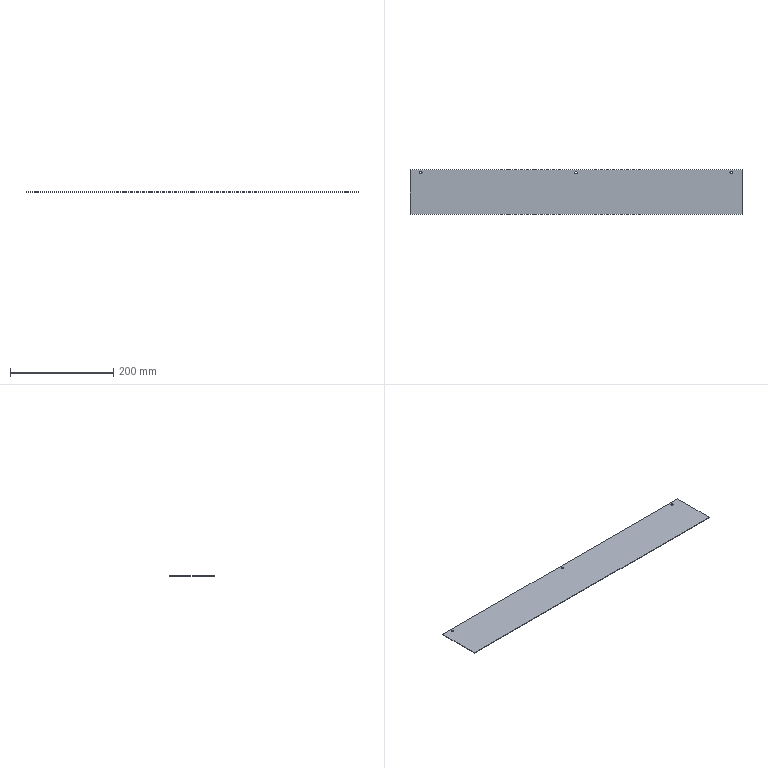Part | SolidWorks | features Cut 1, Extrusion 1 | 1 solid | 12 faces | box 642 x 87 x 1 mm | volume 55806 mm3 | cylinder 6 | plane 6 | commonest cylinder face diameters 4.5 x6
STEP:
#1=CARTESIAN_POINT('',(297.75,37.5,-0.5));
#2=VERTEX_POINT('',#1);
#3=CARTESIAN_POINT('',(302.25,37.5,-0.5));
#4=VERTEX_POINT('',#3);
#5=CARTESIAN_POINT('',(300.,37.5,-0.5));
#6=DIRECTION('',(0.,0.,1.));
#7=DIRECTION('',(-1.,0.,0.));
#8=AXIS2_PLACEMENT_3D('',#5,#6,#7);
#9=CIRCLE('',#8,2.25);
#10=EDGE_CURVE('',#2,#4,#9,.T.);
#11=ORIENTED_EDGE('',*,*,#10,.F.);
#12=CARTESIAN_POINT('',(297.75,37.5,0.5));
#13=VERTEX_POINT('',#12);
#14=CARTESIAN_POINT('',(297.75,37.5,-0.5));
#15=DIRECTION('',(0.,0.,1.));
#16=VECTOR('',#15,1000.);
#17=LINE('',#14,#16);
#18=EDGE_CURVE('',#2,#13,#17,.T.);
#19=ORIENTED_EDGE('',*,*,#18,.T.);
#20=CARTESIAN_POINT('',(302.25,37.5,0.5));
#21=VERTEX_POINT('',#20);
#22=CARTESIAN_POINT('',(300.,37.5,0.5));
#23=DIRECTION('',(0.,0.,1.));
#24=DIRECTION('',(-1.,0.,0.));
#25=AXIS2_PLACEMENT_3D('',#22,#23,#24);
#26=CIRCLE('',#25,2.25);
#27=EDGE_CURVE('',#13,#21,#26,.T.);
#28=ORIENTED_EDGE('',*,*,#27,.T.);
#29=CARTESIAN_POINT('',(302.25,37.5,-0.5));
#30=DIRECTION('',(0.,0.,1.));
#31=VECTOR('',#30,1000.);
#32=LINE('',#29,#31);
#33=EDGE_CURVE('',#4,#21,#32,.T.);
#34=ORIENTED_EDGE('',*,*,#33,.F.);
#35=EDGE_LOOP('',(#11,#19,#28,#34));
#36=FACE_OUTER_BOUND('',#35,.T.);
#37=CARTESIAN_POINT('',(300.,37.5,-0.5));
#38=DIRECTION('',(0.,0.,1.));
#39=DIRECTION('',(1.,0.,0.));
#40=AXIS2_PLACEMENT_3D('',#37,#38,#39);
#41=CYLINDRICAL_SURFACE('',#40,2.25);
#42=ADVANCED_FACE('',(#36),#41,.F.);
#43=CARTESIAN_POINT('',(-2.25,37.5,-0.5));
#44=VERTEX_POINT('',#43);
#45=CARTESIAN_POINT('',(2.25,37.5,-0.5));
#46=VERTEX_POINT('',#45);
#47=CARTESIAN_POINT('',(0.,37.5,-0.5));
#48=DIRECTION('',(0.,0.,1.));
#49=DIRECTION('',(1.,0.,0.));
#50=AXIS2_PLACEMENT_3D('',#47,#48,#49);
#51=CIRCLE('',#50,2.25);
#52=EDGE_CURVE('',#44,#46,#51,.T.);
#53=ORIENTED_EDGE('',*,*,#52,.F.);
#54=CARTESIAN_POINT('',(-2.25,37.5,0.5));
#55=VERTEX_POINT('',#54);
#56=CARTESIAN_POINT('',(-2.25,37.5,-0.5));
#57=DIRECTION('',(0.,0.,1.));
#58=VECTOR('',#57,1000.);
#59=LINE('',#56,#58);
#60=EDGE_CURVE('',#44,#55,#59,.T.);
#61=ORIENTED_EDGE('',*,*,#60,.T.);
#62=CARTESIAN_POINT('',(2.25,37.5,0.5));
#63=VERTEX_POINT('',#62);
#64=CARTESIAN_POINT('',(0.,37.5,0.5));
#65=DIRECTION('',(0.,0.,1.));
#66=DIRECTION('',(1.,0.,0.));
#67=AXIS2_PLACEMENT_3D('',#64,#65,#66);
#68=CIRCLE('',#67,2.25);
#69=EDGE_CURVE('',#55,#63,#68,.T.);
#70=ORIENTED_EDGE('',*,*,#69,.T.);
#71=CARTESIAN_POINT('',(2.25,37.5,-0.5));
#72=DIRECTION('',(0.,0.,1.));
#73=VECTOR('',#72,1000.);
#74=LINE('',#71,#73);
#75=EDGE_CURVE('',#46,#63,#74,.T.);
#76=ORIENTED_EDGE('',*,*,#75,.F.);
#77=EDGE_LOOP('',(#53,#61,#70,#76));
#78=FACE_OUTER_BOUND('',#77,.T.);
#79=CARTESIAN_POINT('',(0.,37.5,-0.5));
#80=DIRECTION('',(0.,0.,1.));
#81=DIRECTION('',(1.,0.,0.));
#82=AXIS2_PLACEMENT_3D('',#79,#80,#81);
#83=CYLINDRICAL_SURFACE('',#82,2.25);
#84=ADVANCED_FACE('',(#78),#83,.F.);
#85=CARTESIAN_POINT('',(-302.25,37.5,-0.5));
#86=VERTEX_POINT('',#85);
#87=CARTESIAN_POINT('',(-297.75,37.5,-0.5));
#88=VERTEX_POINT('',#87);
#89=CARTESIAN_POINT('',(-300.,37.5,-0.5));
#90=DIRECTION('',(0.,0.,1.));
#91=DIRECTION('',(1.,0.,0.));
#92=AXIS2_PLACEMENT_3D('',#89,#90,#91);
#93=CIRCLE('',#92,2.25);
#94=EDGE_CURVE('',#86,#88,#93,.T.);
#95=ORIENTED_EDGE('',*,*,#94,.F.);
#96=CARTESIAN_POINT('',(-302.25,37.5,0.5));
#97=VERTEX_POINT('',#96);
#98=CARTESIAN_POINT('',(-302.25,37.5,-0.5));
#99=DIRECTION('',(0.,0.,1.));
#100=VECTOR('',#99,1000.);
#101=LINE('',#98,#100);
#102=EDGE_CURVE('',#86,#97,#101,.T.);
#103=ORIENTED_EDGE('',*,*,#102,.T.);
#104=CARTESIAN_POINT('',(-297.75,37.5,0.5));
#105=VERTEX_POINT('',#104);
#106=CARTESIAN_POINT('',(-300.,37.5,0.5));
#107=DIRECTION('',(0.,0.,1.));
#108=DIRECTION('',(1.,0.,0.));
#109=AXIS2_PLACEMENT_3D('',#106,#107,#108);
#110=CIRCLE('',#109,2.25);
#111=EDGE_CURVE('',#97,#105,#110,.T.);
#112=ORIENTED_EDGE('',*,*,#111,.T.);
#113=CARTESIAN_POINT('',(-297.75,37.5,-0.5));
#114=DIRECTION('',(0.,0.,1.));
#115=VECTOR('',#114,1000.);
#116=LINE('',#113,#115);
#117=EDGE_CURVE('',#88,#105,#116,.T.);
#118=ORIENTED_EDGE('',*,*,#117,.F.);
#119=EDGE_LOOP('',(#95,#103,#112,#118));
#120=FACE_OUTER_BOUND('',#119,.T.);
#121=CARTESIAN_POINT('',(-300.,37.5,-0.5));
#122=DIRECTION('',(0.,0.,1.));
#123=DIRECTION('',(1.,0.,0.));
#124=AXIS2_PLACEMENT_3D('',#121,#122,#123);
#125=CYLINDRICAL_SURFACE('',#124,2.25);
#126=ADVANCED_FACE('',(#120),#125,.F.);
#127=CARTESIAN_POINT('',(-321.,-43.5,-0.5));
#128=VERTEX_POINT('',#127);
#129=CARTESIAN_POINT('',(-321.,-43.5,0.5));
#130=VERTEX_POINT('',#129);
#131=CARTESIAN_POINT('',(-321.,-43.5,-0.5));
#132=DIRECTION('',(0.,0.,1.));
#133=VECTOR('',#132,1000.);
#134=LINE('',#131,#133);
#135=EDGE_CURVE('',#128,#130,#134,.T.);
#136=ORIENTED_EDGE('',*,*,#135,.T.);
#137=CARTESIAN_POINT('',(-321.,43.5,0.5));
#138=VERTEX_POINT('',#137);
#139=CARTESIAN_POINT('',(-321.,43.5,0.5));
#140=DIRECTION('',(0.,-1.,0.));
#141=VECTOR('',#140,1000.);
#142=LINE('',#139,#141);
#143=EDGE_CURVE('',#138,#130,#142,.T.);
#144=ORIENTED_EDGE('',*,*,#143,.F.);
#145=CARTESIAN_POINT('',(-321.,43.5,-0.5));
#146=VERTEX_POINT('',#145);
#147=CARTESIAN_POINT('',(-321.,43.5,-0.5));
#148=DIRECTION('',(0.,0.,1.));
#149=VECTOR('',#148,1000.);
#150=LINE('',#147,#149);
#151=EDGE_CURVE('',#146,#138,#150,.T.);
#152=ORIENTED_EDGE('',*,*,#151,.F.);
#153=CARTESIAN_POINT('',(-321.,43.5,-0.5));
#154=DIRECTION('',(0.,-1.,0.));
#155=VECTOR('',#154,1000.);
#156=LINE('',#153,#155);
#157=EDGE_CURVE('',#146,#128,#156,.T.);
#158=ORIENTED_EDGE('',*,*,#157,.T.);
#159=EDGE_LOOP('',(#136,#144,#152,#158));
#160=FACE_OUTER_BOUND('',#159,.T.);
#161=CARTESIAN_POINT('',(-321.,43.5,-0.5));
#162=DIRECTION('',(1.,0.,0.));
#163=DIRECTION('',(0.,0.,-1.));
#164=AXIS2_PLACEMENT_3D('',#161,#162,#163);
#165=PLANE('',#164);
#166=ADVANCED_FACE('',(#160),#165,.F.);
#167=CARTESIAN_POINT('',(300.,37.5,0.5));
#168=DIRECTION('',(0.,0.,1.));
#169=DIRECTION('',(-1.,0.,0.));
#170=AXIS2_PLACEMENT_3D('',#167,#168,#169);
#171=CIRCLE('',#170,2.25);
#172=EDGE_CURVE('',#21,#13,#171,.T.);
#173=ORIENTED_EDGE('',*,*,#172,.F.);
#174=ORIENTED_EDGE('',*,*,#27,.F.);
#175=EDGE_LOOP('',(#173,#174));
#176=FACE_BOUND('',#175,.T.);
#177=CARTESIAN_POINT('',(0.,37.5,0.5));
#178=DIRECTION('',(0.,0.,1.));
#179=DIRECTION('',(1.,0.,0.));
#180=AXIS2_PLACEMENT_3D('',#177,#178,#179);
#181=CIRCLE('',#180,2.25);
#182=EDGE_CURVE('',#63,#55,#181,.T.);
#183=ORIENTED_EDGE('',*,*,#182,.F.);
#184=ORIENTED_EDGE('',*,*,#69,.F.);
#185=EDGE_LOOP('',(#183,#184));
#186=FACE_BOUND('',#185,.T.);
#187=CARTESIAN_POINT('',(-300.,37.5,0.5));
#188=DIRECTION('',(0.,0.,1.));
#189=DIRECTION('',(1.,0.,0.));
#190=AXIS2_PLACEMENT_3D('',#187,#188,#189);
#191=CIRCLE('',#190,2.25);
#192=EDGE_CURVE('',#105,#97,#191,.T.);
#193=ORIENTED_EDGE('',*,*,#192,.F.);
#194=ORIENTED_EDGE('',*,*,#111,.F.);
#195=EDGE_LOOP('',(#193,#194));
#196=FACE_BOUND('',#195,.T.);
#197=CARTESIAN_POINT('',(321.,-43.5,0.5));
#198=VERTEX_POINT('',#197);
#199=CARTESIAN_POINT('',(-321.,-43.5,0.5));
#200=DIRECTION('',(1.,0.,0.));
#201=VECTOR('',#200,1000.);
#202=LINE('',#199,#201);
#203=EDGE_CURVE('',#130,#198,#202,.T.);
#204=ORIENTED_EDGE('',*,*,#203,.T.);
#205=CARTESIAN_POINT('',(321.,43.5,0.5));
#206=VERTEX_POINT('',#205);
#207=CARTESIAN_POINT('',(321.,43.5,0.5));
#208=DIRECTION('',(0.,-1.,0.));
#209=VECTOR('',#208,1000.);
#210=LINE('',#207,#209);
#211=EDGE_CURVE('',#206,#198,#210,.T.);
#212=ORIENTED_EDGE('',*,*,#211,.F.);
#213=CARTESIAN_POINT('',(-321.,43.5,0.5));
#214=DIRECTION('',(1.,0.,0.));
#215=VECTOR('',#214,1000.);
#216=LINE('',#213,#215);
#217=EDGE_CURVE('',#138,#206,#216,.T.);
#218=ORIENTED_EDGE('',*,*,#217,.F.);
#219=ORIENTED_EDGE('',*,*,#143,.T.);
#220=EDGE_LOOP('',(#204,#212,#218,#219));
#221=FACE_OUTER_BOUND('',#220,.T.);
#222=CARTESIAN_POINT('',(-321.,43.5,0.5));
#223=DIRECTION('',(0.,0.,-1.));
#224=DIRECTION('',(-1.,0.,0.));
#225=AXIS2_PLACEMENT_3D('',#222,#223,#224);
#226=PLANE('',#225);
#227=ADVANCED_FACE('',(#176,#186,#196,#221),#226,.F.);
#228=CARTESIAN_POINT('',(321.,-43.5,-0.5));
#229=VERTEX_POINT('',#228);
#230=CARTESIAN_POINT('',(321.,-43.5,-0.5));
#231=DIRECTION('',(0.,0.,-1.));
#232=VECTOR('',#231,1000.);
#233=LINE('',#230,#232);
#234=EDGE_CURVE('',#198,#229,#233,.T.);
#235=ORIENTED_EDGE('',*,*,#234,.T.);
#236=CARTESIAN_POINT('',(321.,43.5,-0.5));
#237=VERTEX_POINT('',#236);
#238=CARTESIAN_POINT('',(321.,43.5,-0.5));
#239=DIRECTION('',(0.,-1.,0.));
#240=VECTOR('',#239,1000.);
#241=LINE('',#238,#240);
#242=EDGE_CURVE('',#237,#229,#241,.T.);
#243=ORIENTED_EDGE('',*,*,#242,.F.);
#244=CARTESIAN_POINT('',(321.,43.5,-0.5));
#245=DIRECTION('',(0.,0.,-1.));
#246=VECTOR('',#245,1000.);
#247=LINE('',#244,#246);
#248=EDGE_CURVE('',#206,#237,#247,.T.);
#249=ORIENTED_EDGE('',*,*,#248,.F.);
#250=ORIENTED_EDGE('',*,*,#211,.T.);
#251=EDGE_LOOP('',(#235,#243,#249,#250));
#252=FACE_OUTER_BOUND('',#251,.T.);
#253=CARTESIAN_POINT('',(321.,43.5,-0.5));
#254=DIRECTION('',(-1.,0.,0.));
#255=DIRECTION('',(0.,0.,1.));
#256=AXIS2_PLACEMENT_3D('',#253,#254,#255);
#257=PLANE('',#256);
#258=ADVANCED_FACE('',(#252),#257,.F.);
#259=CARTESIAN_POINT('',(300.,37.5,-0.5));
#260=DIRECTION('',(0.,0.,1.));
#261=DIRECTION('',(-1.,0.,0.));
#262=AXIS2_PLACEMENT_3D('',#259,#260,#261);
#263=CIRCLE('',#262,2.25);
#264=EDGE_CURVE('',#4,#2,#263,.T.);
#265=ORIENTED_EDGE('',*,*,#264,.T.);
#266=ORIENTED_EDGE('',*,*,#10,.T.);
#267=EDGE_LOOP('',(#265,#266));
#268=FACE_BOUND('',#267,.T.);
#269=CARTESIAN_POINT('',(0.,37.5,-0.5));
#270=DIRECTION('',(0.,0.,1.));
#271=DIRECTION('',(1.,0.,0.));
#272=AXIS2_PLACEMENT_3D('',#269,#270,#271);
#273=CIRCLE('',#272,2.25);
#274=EDGE_CURVE('',#46,#44,#273,.T.);
#275=ORIENTED_EDGE('',*,*,#274,.T.);
#276=ORIENTED_EDGE('',*,*,#52,.T.);
#277=EDGE_LOOP('',(#275,#276));
#278=FACE_BOUND('',#277,.T.);
#279=CARTESIAN_POINT('',(-300.,37.5,-0.5));
#280=DIRECTION('',(0.,0.,1.));
#281=DIRECTION('',(1.,0.,0.));
#282=AXIS2_PLACEMENT_3D('',#279,#280,#281);
#283=CIRCLE('',#282,2.25);
#284=EDGE_CURVE('',#88,#86,#283,.T.);
#285=ORIENTED_EDGE('',*,*,#284,.T.);
#286=ORIENTED_EDGE('',*,*,#94,.T.);
#287=EDGE_LOOP('',(#285,#286));
#288=FACE_BOUND('',#287,.T.);
#289=CARTESIAN_POINT('',(-321.,-43.5,-0.5));
#290=DIRECTION('',(-1.,0.,0.));
#291=VECTOR('',#290,1000.);
#292=LINE('',#289,#291);
#293=EDGE_CURVE('',#229,#128,#292,.T.);
#294=ORIENTED_EDGE('',*,*,#293,.T.);
#295=ORIENTED_EDGE('',*,*,#157,.F.);
#296=CARTESIAN_POINT('',(-321.,43.5,-0.5));
#297=DIRECTION('',(-1.,0.,0.));
#298=VECTOR('',#297,1000.);
#299=LINE('',#296,#298);
#300=EDGE_CURVE('',#237,#146,#299,.T.);
#301=ORIENTED_EDGE('',*,*,#300,.F.);
#302=ORIENTED_EDGE('',*,*,#242,.T.);
#303=EDGE_LOOP('',(#294,#295,#301,#302));
#304=FACE_OUTER_BOUND('',#303,.T.);
#305=CARTESIAN_POINT('',(-321.,43.5,-0.5));
#306=DIRECTION('',(0.,0.,1.));
#307=DIRECTION('',(1.,0.,0.));
#308=AXIS2_PLACEMENT_3D('',#305,#306,#307);
#309=PLANE('',#308);
#310=ADVANCED_FACE('',(#268,#278,#288,#304),#309,.F.);
#311=ORIENTED_EDGE('',*,*,#151,.T.);
#312=ORIENTED_EDGE('',*,*,#217,.T.);
#313=ORIENTED_EDGE('',*,*,#248,.T.);
#314=ORIENTED_EDGE('',*,*,#300,.T.);
#315=EDGE_LOOP('',(#311,#312,#313,#314));
#316=FACE_OUTER_BOUND('',#315,.T.);
#317=CARTESIAN_POINT('',(-321.,43.5,0.5));
#318=DIRECTION('',(0.,1.,0.));
#319=DIRECTION('',(0.,0.,1.));
#320=AXIS2_PLACEMENT_3D('',#317,#318,#319);
#321=PLANE('',#320);
#322=ADVANCED_FACE('',(#316),#321,.T.);
#323=ORIENTED_EDGE('',*,*,#135,.F.);
#324=ORIENTED_EDGE('',*,*,#293,.F.);
#325=ORIENTED_EDGE('',*,*,#234,.F.);
#326=ORIENTED_EDGE('',*,*,#203,.F.);
#327=EDGE_LOOP('',(#323,#324,#325,#326));
#328=FACE_OUTER_BOUND('',#327,.T.);
#329=CARTESIAN_POINT('',(-321.,-43.5,0.5));
#330=DIRECTION('',(0.,1.,0.));
#331=DIRECTION('',(0.,0.,1.));
#332=AXIS2_PLACEMENT_3D('',#329,#330,#331);
#333=PLANE('',#332);
#334=ADVANCED_FACE('',(#328),#333,.F.);
#335=ORIENTED_EDGE('',*,*,#102,.F.);
#336=ORIENTED_EDGE('',*,*,#284,.F.);
#337=ORIENTED_EDGE('',*,*,#117,.T.);
#338=ORIENTED_EDGE('',*,*,#192,.T.);
#339=EDGE_LOOP('',(#335,#336,#337,#338));
#340=FACE_OUTER_BOUND('',#339,.T.);
#341=CARTESIAN_POINT('',(-300.,37.5,-0.5));
#342=DIRECTION('',(0.,0.,1.));
#343=DIRECTION('',(1.,0.,0.));
#344=AXIS2_PLACEMENT_3D('',#341,#342,#343);
#345=CYLINDRICAL_SURFACE('',#344,2.25);
#346=ADVANCED_FACE('',(#340),#345,.F.);
#347=ORIENTED_EDGE('',*,*,#60,.F.);
#348=ORIENTED_EDGE('',*,*,#274,.F.);
#349=ORIENTED_EDGE('',*,*,#75,.T.);
#350=ORIENTED_EDGE('',*,*,#182,.T.);
#351=EDGE_LOOP('',(#347,#348,#349,#350));
#352=FACE_OUTER_BOUND('',#351,.T.);
#353=CARTESIAN_POINT('',(0.,37.5,-0.5));
#354=DIRECTION('',(0.,0.,1.));
#355=DIRECTION('',(1.,0.,0.));
#356=AXIS2_PLACEMENT_3D('',#353,#354,#355);
#357=CYLINDRICAL_SURFACE('',#356,2.25);
#358=ADVANCED_FACE('',(#352),#357,.F.);
#359=ORIENTED_EDGE('',*,*,#18,.F.);
#360=ORIENTED_EDGE('',*,*,#264,.F.);
#361=ORIENTED_EDGE('',*,*,#33,.T.);
#362=ORIENTED_EDGE('',*,*,#172,.T.);
#363=EDGE_LOOP('',(#359,#360,#361,#362));
#364=FACE_OUTER_BOUND('',#363,.T.);
#365=CARTESIAN_POINT('',(300.,37.5,-0.5));
#366=DIRECTION('',(0.,0.,1.));
#367=DIRECTION('',(1.,0.,0.));
#368=AXIS2_PLACEMENT_3D('',#365,#366,#367);
#369=CYLINDRICAL_SURFACE('',#368,2.25);
#370=ADVANCED_FACE('',(#364),#369,.F.);
#371=CLOSED_SHELL('',(#42,#84,#126,#166,#227,#258,#310,#322,#334,#346,#358,#370));
#372=MANIFOLD_SOLID_BREP('',#371);
#373=CARTESIAN_POINT('',(0.,0.,0.));
#374=DIRECTION('',(0.,0.,1.));
#375=DIRECTION('',(1.,0.,0.));
#376=AXIS2_PLACEMENT_3D('',#373,#374,#375);
#377=(LENGTH_UNIT()NAMED_UNIT(*)SI_UNIT(.MILLI.,.METRE.));
#378=UNCERTAINTY_MEASURE_WITH_UNIT(LENGTH_MEASURE(0.00001),#377,'','');
#379=(NAMED_UNIT(*)PLANE_ANGLE_UNIT()SI_UNIT($,.RADIAN.));
#380=(NAMED_UNIT(*)SI_UNIT($,.STERADIAN.)SOLID_ANGLE_UNIT());
#381=(GEOMETRIC_REPRESENTATION_CONTEXT(3)GLOBAL_UNCERTAINTY_ASSIGNED_CONTEXT((#378))GLOBAL_UNIT_ASSIGNED_CONTEXT((#377,#379,#380))REPRESENTATION_CONTEXT('',''));
#382=ADVANCED_BREP_SHAPE_REPRESENTATION('',(#372,#376),#381);